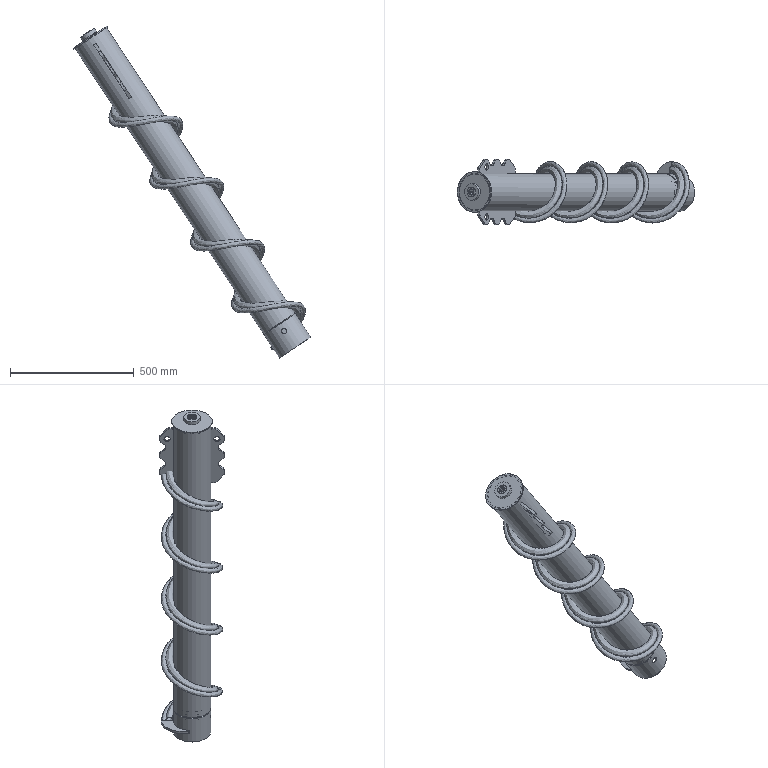Part | STEP file | HL4GZ-1.862.030 (right spiral roller shaft) | 11 solids | 156 faces | box 960.116 x 266 x 1342 mm | volume 5047297 mm3 | plane 73 | cylinder 73 | cone 6 | spline 4 | commonest cylinder face diameters 0.4 x12 40 x12 6 x11 21.4 x6 25.3 x6 145 x5